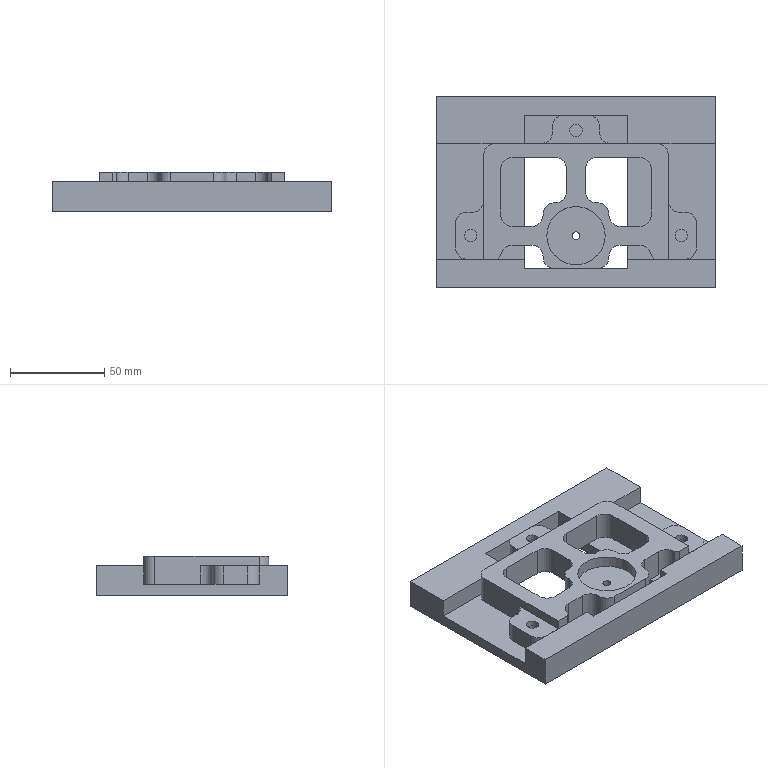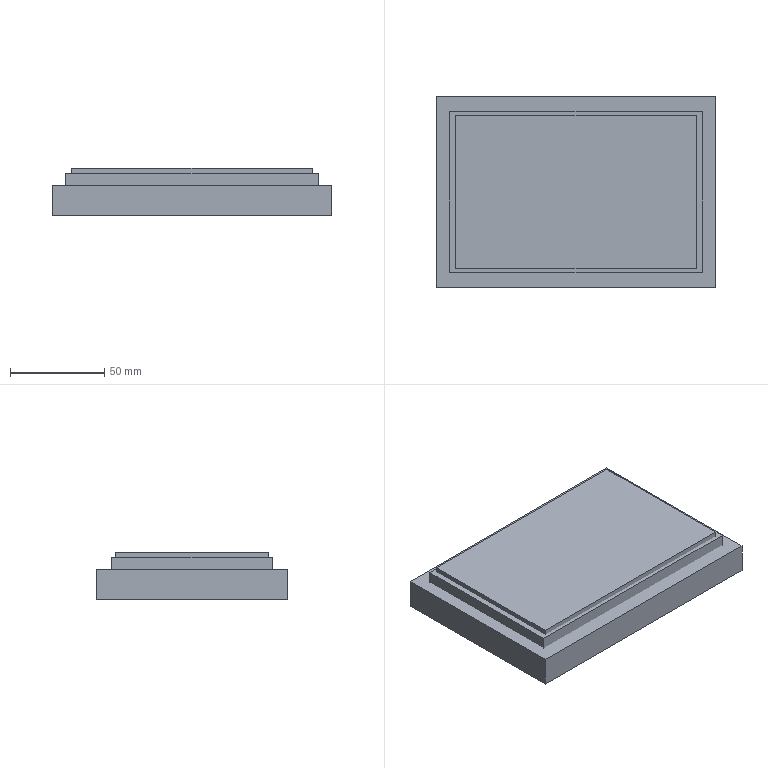CAM job | NX | 3-axis milling, drilling | part box 148 x 101.5 x 21 mm | stock box 148 x 101.5 x 25 mm
Tools:
number,name,description,diameter,corner_radius,flute_length,length,flutes
1,D63,Milling Tool-5 Parameters,63.0,0.0,50.0,75.0,2
4,D10,Milling Tool-5 Parameters,10.0,0.0,50.0,75.0,2
14,D10JING,Milling Tool-5 Parameters,10.0,0.0,50.0,75.0,2
1,D6A45,Milling Tool-5 Parameters,6.0,0.0,3.0,3.0,2
12,4.2ZT,Drilling Tool,4.2,0.0,35.0,50.0,2
13,6.6ZT,Drilling Tool,6.6,0.0,35.0,50.0,2
16,D6,Milling Tool-5 Parameters,6.0,0.0,50.0,75.0,2
17,D4,Milling Tool-5 Parameters,4.0,0.0,50.0,75.0,2
Operations:
program,operation,operation_type,tool,method,geometry_group,spindle_rpm,surface_speed,feed_per_tooth,feed_cut,feed_plunge,cut_length_mm,path_length_mm,cut_time_min,machine_time_min
1夹粗,FLOOR_WALL,VolumeBased25DMillingOperation,D63,METHOD,A,6500.0,1286.0,0.1154,1500.0,100.0,663.297,715.297,0.4422,0.4474
1夹粗,ADAPTIVE_MILLING,CavityMilling,D10,METHOD,A,9500.0,298.0,0.1579,3000.0,1000.0,13359.673,14241.465,6.6,6.689
1夹精,FLOOR_WALL_COPY,VolumeBased25DMillingOperation,D10,METHOD,A,9500.0,298.0,0.1053,2000.0,1000.0,4367.086,4933.216,2.215,2.272
1夹精,DRILLING,Operation,D6A45,METHOD,A,5000.0,94.0,0.025,250.0,0.0,16.0,302.431,0.064,0.0926
1夹精,DRILLING_COPY,Operation,4.2ZT,METHOD,A,2000.0,26.0,0.0625,250.0,0.0,13.262,98.524,0.053,0.0616
1夹精,DRILLING_COPY_COPY,Operation,6.6ZT,METHOD,A,2000.0,41.0,0.0625,250.0,0.0,29.049,292.603,0.1162,0.1425
1夹精,ZLEVEL_PROFILE_COPY_1,ZLevelMilling,D10,METHOD,A,9500.0,298.0,0.1158,2200.0,1000.0,4749.827,5143.333,2.199,2.239
1夹精,ZLEVEL_PROFILE,ZLevelMilling,D10,METHOD,A,9500.0,298.0,0.1158,2200.0,1000.0,8891.384,9023.173,4.059,4.073
1夹精,ZLEVEL_PROFILE_COPY,ZLevelMilling,D10JING,METHOD,A,9500.0,298.0,0.0632,1200.0,1000.0,199.609,471.619,0.167,0.1942
1夹精,FLOOR_WALL_COPY_COPY,VolumeBased25DMillingOperation,D10JING,METHOD,A,9500.0,298.0,0.0526,1000.0,1000.0,2305.271,3080.155,2.305,2.387
1夹精,ZLEVEL_PROFILE_COPY_COPY,ZLevelMilling,D10JING,METHOD,A,9500.0,298.0,0.0632,1200.0,1000.0,435.492,537.492,0.3633,0.3735
1夹精,ZLEVEL_PROFILE_1,ZLevelMilling,D6A45,METHOD,A,9500.0,179.0,0.0658,1250.0,100.0,926.462,2308.49,0.7412,0.8794
2夹,FLOOR_WALL_COPY_1,VolumeBased25DMillingOperation,D10,METHOD,B,9505.0,298.0,0.1315,2500.0,100.0,9741.988,10436.076,3.897,3.966
2夹,FLOOR_WALL_COPY_1_COPY,VolumeBased25DMillingOperation,D10,METHOD,B,9505.0,298.0,0.1157,2200.0,100.0,12189.04,12739.336,5.54,5.596
2夹,FLOOR_WALL_COPY_1_COPY_COPY,VolumeBased25DMillingOperation,D10,METHOD,B,9505.0,298.0,0.1157,2200.0,100.0,1162.934,1788.651,0.5286,0.5912
2夹,FLOOR_WALL_COPY_COPY_COPY,VolumeBased25DMillingOperation,D10JING,METHOD,B,9500.0,298.0,0.0526,1000.0,1000.0,2106.958,2894.209,2.107,2.19
2夹,ZLEVEL_PROFILE_COPY_COPY_COPY,ZLevelMilling,D10JING,METHOD,B,9500.0,298.0,0.0632,1200.0,1000.0,116.095,188.095,0.097,0.1042
2夹,HOLE_MILLING,CylinderMilling,D6,METHOD,B,9500.0,179.0,0.0763,1450.0,100.0,759.043,1152.335,0.5235,0.5628
2夹,ZLEVEL_PROFILE_1_COPY,ZLevelMilling,D6A45,METHOD,B,9500.0,179.0,0.0658,1250.0,100.0,910.561,1911.525,0.7284,0.8285
夹具钳口,ADAPTIVE_MILLING_COPY,CavityMilling,D10,METHOD,C,9500.0,298.0,0.1579,3000.0,1000.0,14975.053,15157.944,5.72,5.738
夹具钳口,FLOOR_WALL_COPY_COPY_COPY_1,VolumeBased25DMillingOperation,D10JING,METHOD,C,9500.0,298.0,0.0526,1000.0,1000.0,1902.45,2431.478,1.903,1.96
夹具钳口,ZLEVEL_PROFILE_COPY_COPY_1,ZLevelMilling,D10JING,METHOD,C,9500.0,298.0,0.0632,1200.0,1000.0,206.249,298.249,0.1721,0.1813
夹具钳口,PLANAR_MILL_COPY,PlanarMilling,D10JING,METHOD,C,9486.0,298.0,0.0633,1200.0,1000.0,829.74,915.74,0.6923,0.7009
夹具钳口,ZLEVEL_PROFILE_2,ZLevelMilling,D4,METHOD,C,9500.0,119.0,0.0632,1200.0,100.0,1279.55,2610.907,1.066,1.199